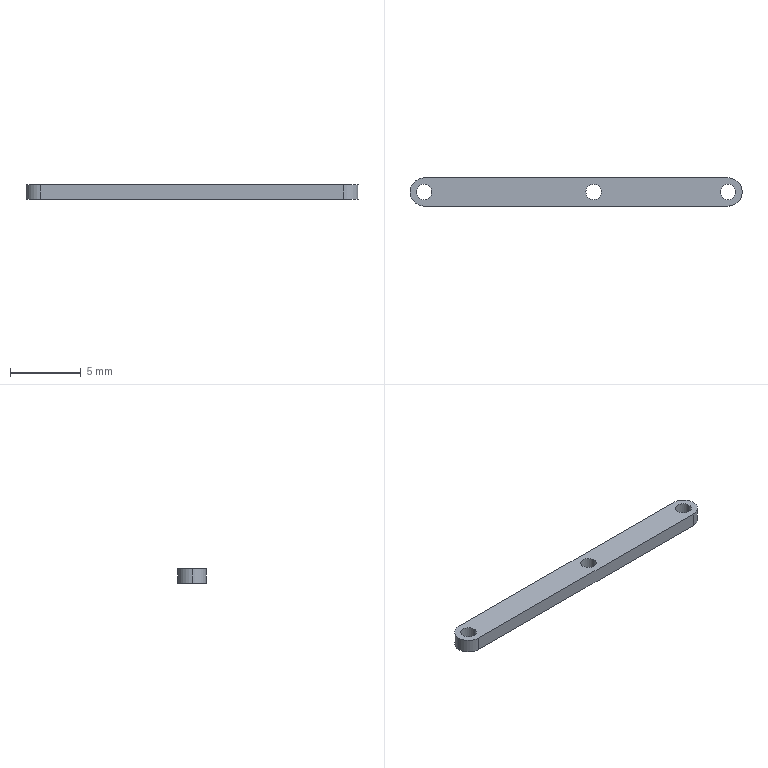Part | SolidWorks | features Extrusion 1, ICE 1 | 1 solid | 13 faces | box 23.5 x 2 x 1 mm | volume 43.291 mm3 | cylinder 9 | plane 4 | commonest cylinder face diameters 1.1 x6 2 x3
STEP:
#1=CARTESIAN_POINT('',(0.7,0.,0.5));
#2=VERTEX_POINT('',#1);
#3=CARTESIAN_POINT('',(1.8,0.,0.5));
#4=VERTEX_POINT('',#3);
#5=CARTESIAN_POINT('',(1.25,0.,0.5));
#6=DIRECTION('',(0.,0.,1.));
#7=DIRECTION('',(1.,0.,0.));
#8=AXIS2_PLACEMENT_3D('',#5,#6,#7);
#9=CIRCLE('',#8,0.55);
#10=EDGE_CURVE('',#2,#4,#9,.T.);
#11=ORIENTED_EDGE('',*,*,#10,.T.);
#12=CARTESIAN_POINT('',(1.8,0.,-0.5));
#13=VERTEX_POINT('',#12);
#14=CARTESIAN_POINT('',(1.8,0.,0.5));
#15=DIRECTION('',(0.,0.,-1.));
#16=VECTOR('',#15,1000.);
#17=LINE('',#14,#16);
#18=EDGE_CURVE('',#4,#13,#17,.T.);
#19=ORIENTED_EDGE('',*,*,#18,.T.);
#20=CARTESIAN_POINT('',(0.7,0.,-0.5));
#21=VERTEX_POINT('',#20);
#22=CARTESIAN_POINT('',(1.25,0.,-0.5));
#23=DIRECTION('',(0.,0.,1.));
#24=DIRECTION('',(1.,0.,0.));
#25=AXIS2_PLACEMENT_3D('',#22,#23,#24);
#26=CIRCLE('',#25,0.55);
#27=EDGE_CURVE('',#21,#13,#26,.T.);
#28=ORIENTED_EDGE('',*,*,#27,.F.);
#29=CARTESIAN_POINT('',(0.7,0.,0.5));
#30=DIRECTION('',(0.,0.,-1.));
#31=VECTOR('',#30,1000.);
#32=LINE('',#29,#31);
#33=EDGE_CURVE('',#2,#21,#32,.T.);
#34=ORIENTED_EDGE('',*,*,#33,.F.);
#35=EDGE_LOOP('',(#11,#19,#28,#34));
#36=FACE_OUTER_BOUND('',#35,.T.);
#37=CARTESIAN_POINT('',(1.25,0.,0.5));
#38=DIRECTION('',(0.,0.,-1.));
#39=DIRECTION('',(-1.,0.,0.));
#40=AXIS2_PLACEMENT_3D('',#37,#38,#39);
#41=CYLINDRICAL_SURFACE('',#40,0.55);
#42=ADVANCED_FACE('',(#36),#41,.F.);
#43=CARTESIAN_POINT('',(10.2,0.,0.5));
#44=VERTEX_POINT('',#43);
#45=CARTESIAN_POINT('',(11.3,0.,0.5));
#46=VERTEX_POINT('',#45);
#47=CARTESIAN_POINT('',(10.75,0.,0.5));
#48=DIRECTION('',(0.,0.,1.));
#49=DIRECTION('',(1.,0.,0.));
#50=AXIS2_PLACEMENT_3D('',#47,#48,#49);
#51=CIRCLE('',#50,0.55);
#52=EDGE_CURVE('',#44,#46,#51,.T.);
#53=ORIENTED_EDGE('',*,*,#52,.T.);
#54=CARTESIAN_POINT('',(11.3,0.,-0.5));
#55=VERTEX_POINT('',#54);
#56=CARTESIAN_POINT('',(11.3,0.,0.5));
#57=DIRECTION('',(0.,0.,-1.));
#58=VECTOR('',#57,1000.);
#59=LINE('',#56,#58);
#60=EDGE_CURVE('',#46,#55,#59,.T.);
#61=ORIENTED_EDGE('',*,*,#60,.T.);
#62=CARTESIAN_POINT('',(10.2,0.,-0.5));
#63=VERTEX_POINT('',#62);
#64=CARTESIAN_POINT('',(10.75,0.,-0.5));
#65=DIRECTION('',(0.,0.,1.));
#66=DIRECTION('',(1.,0.,0.));
#67=AXIS2_PLACEMENT_3D('',#64,#65,#66);
#68=CIRCLE('',#67,0.55);
#69=EDGE_CURVE('',#63,#55,#68,.T.);
#70=ORIENTED_EDGE('',*,*,#69,.F.);
#71=CARTESIAN_POINT('',(10.2,0.,0.5));
#72=DIRECTION('',(0.,0.,-1.));
#73=VECTOR('',#72,1000.);
#74=LINE('',#71,#73);
#75=EDGE_CURVE('',#44,#63,#74,.T.);
#76=ORIENTED_EDGE('',*,*,#75,.F.);
#77=EDGE_LOOP('',(#53,#61,#70,#76));
#78=FACE_OUTER_BOUND('',#77,.T.);
#79=CARTESIAN_POINT('',(10.75,0.,0.5));
#80=DIRECTION('',(0.,0.,-1.));
#81=DIRECTION('',(-1.,0.,0.));
#82=AXIS2_PLACEMENT_3D('',#79,#80,#81);
#83=CYLINDRICAL_SURFACE('',#82,0.55);
#84=ADVANCED_FACE('',(#78),#83,.F.);
#85=CARTESIAN_POINT('',(-11.3,0.,0.5));
#86=VERTEX_POINT('',#85);
#87=CARTESIAN_POINT('',(-10.2,0.,0.5));
#88=VERTEX_POINT('',#87);
#89=CARTESIAN_POINT('',(-10.75,0.,0.5));
#90=DIRECTION('',(0.,0.,1.));
#91=DIRECTION('',(1.,0.,0.));
#92=AXIS2_PLACEMENT_3D('',#89,#90,#91);
#93=CIRCLE('',#92,0.55);
#94=EDGE_CURVE('',#86,#88,#93,.T.);
#95=ORIENTED_EDGE('',*,*,#94,.T.);
#96=CARTESIAN_POINT('',(-10.2,0.,-0.5));
#97=VERTEX_POINT('',#96);
#98=CARTESIAN_POINT('',(-10.2,0.,0.5));
#99=DIRECTION('',(0.,0.,-1.));
#100=VECTOR('',#99,1000.);
#101=LINE('',#98,#100);
#102=EDGE_CURVE('',#88,#97,#101,.T.);
#103=ORIENTED_EDGE('',*,*,#102,.T.);
#104=CARTESIAN_POINT('',(-11.3,0.,-0.5));
#105=VERTEX_POINT('',#104);
#106=CARTESIAN_POINT('',(-10.75,0.,-0.5));
#107=DIRECTION('',(0.,0.,1.));
#108=DIRECTION('',(1.,0.,0.));
#109=AXIS2_PLACEMENT_3D('',#106,#107,#108);
#110=CIRCLE('',#109,0.55);
#111=EDGE_CURVE('',#105,#97,#110,.T.);
#112=ORIENTED_EDGE('',*,*,#111,.F.);
#113=CARTESIAN_POINT('',(-11.3,0.,0.5));
#114=DIRECTION('',(0.,0.,-1.));
#115=VECTOR('',#114,1000.);
#116=LINE('',#113,#115);
#117=EDGE_CURVE('',#86,#105,#116,.T.);
#118=ORIENTED_EDGE('',*,*,#117,.F.);
#119=EDGE_LOOP('',(#95,#103,#112,#118));
#120=FACE_OUTER_BOUND('',#119,.T.);
#121=CARTESIAN_POINT('',(-10.75,0.,0.5));
#122=DIRECTION('',(0.,0.,-1.));
#123=DIRECTION('',(-1.,0.,0.));
#124=AXIS2_PLACEMENT_3D('',#121,#122,#123);
#125=CYLINDRICAL_SURFACE('',#124,0.55);
#126=ADVANCED_FACE('',(#120),#125,.F.);
#127=CARTESIAN_POINT('',(-11.75,0.,0.5));
#128=VERTEX_POINT('',#127);
#129=CARTESIAN_POINT('',(-10.75,-1.,0.5));
#130=VERTEX_POINT('',#129);
#131=CARTESIAN_POINT('',(-10.75,0.,0.5));
#132=DIRECTION('',(0.,0.,1.));
#133=DIRECTION('',(1.,0.,0.));
#134=AXIS2_PLACEMENT_3D('',#131,#132,#133);
#135=CIRCLE('',#134,1.);
#136=EDGE_CURVE('',#128,#130,#135,.T.);
#137=ORIENTED_EDGE('',*,*,#136,.F.);
#138=CARTESIAN_POINT('',(-11.75,0.,-0.5));
#139=VERTEX_POINT('',#138);
#140=CARTESIAN_POINT('',(-11.75,0.,0.5));
#141=DIRECTION('',(0.,0.,-1.));
#142=VECTOR('',#141,1000.);
#143=LINE('',#140,#142);
#144=EDGE_CURVE('',#128,#139,#143,.T.);
#145=ORIENTED_EDGE('',*,*,#144,.T.);
#146=CARTESIAN_POINT('',(-10.75,-1.,-0.5));
#147=VERTEX_POINT('',#146);
#148=CARTESIAN_POINT('',(-10.75,0.,-0.5));
#149=DIRECTION('',(0.,0.,1.));
#150=DIRECTION('',(1.,0.,0.));
#151=AXIS2_PLACEMENT_3D('',#148,#149,#150);
#152=CIRCLE('',#151,1.);
#153=EDGE_CURVE('',#139,#147,#152,.T.);
#154=ORIENTED_EDGE('',*,*,#153,.T.);
#155=CARTESIAN_POINT('',(-10.75,-1.,0.5));
#156=DIRECTION('',(0.,0.,-1.));
#157=VECTOR('',#156,1000.);
#158=LINE('',#155,#157);
#159=EDGE_CURVE('',#130,#147,#158,.T.);
#160=ORIENTED_EDGE('',*,*,#159,.F.);
#161=EDGE_LOOP('',(#137,#145,#154,#160));
#162=FACE_OUTER_BOUND('',#161,.T.);
#163=CARTESIAN_POINT('',(-10.75,0.,0.5));
#164=DIRECTION('',(0.,0.,-1.));
#165=DIRECTION('',(-1.,0.,0.));
#166=AXIS2_PLACEMENT_3D('',#163,#164,#165);
#167=CYLINDRICAL_SURFACE('',#166,1.);
#168=ADVANCED_FACE('',(#162),#167,.T.);
#169=ORIENTED_EDGE('',*,*,#52,.F.);
#170=CARTESIAN_POINT('',(10.75,0.,0.5));
#171=DIRECTION('',(0.,0.,1.));
#172=DIRECTION('',(1.,0.,0.));
#173=AXIS2_PLACEMENT_3D('',#170,#171,#172);
#174=CIRCLE('',#173,0.55);
#175=EDGE_CURVE('',#46,#44,#174,.T.);
#176=ORIENTED_EDGE('',*,*,#175,.F.);
#177=EDGE_LOOP('',(#169,#176));
#178=FACE_BOUND('',#177,.T.);
#179=CARTESIAN_POINT('',(-10.75,1.,0.5));
#180=VERTEX_POINT('',#179);
#181=CARTESIAN_POINT('',(-10.75,0.,0.5));
#182=DIRECTION('',(0.,0.,1.));
#183=DIRECTION('',(1.,0.,0.));
#184=AXIS2_PLACEMENT_3D('',#181,#182,#183);
#185=CIRCLE('',#184,1.);
#186=EDGE_CURVE('',#180,#128,#185,.T.);
#187=ORIENTED_EDGE('',*,*,#186,.T.);
#188=ORIENTED_EDGE('',*,*,#136,.T.);
#189=CARTESIAN_POINT('',(10.75,-1.,0.5));
#190=VERTEX_POINT('',#189);
#191=CARTESIAN_POINT('',(-10.75,-1.,0.5));
#192=DIRECTION('',(1.,0.,0.));
#193=VECTOR('',#192,1000.);
#194=LINE('',#191,#193);
#195=EDGE_CURVE('',#130,#190,#194,.T.);
#196=ORIENTED_EDGE('',*,*,#195,.T.);
#197=CARTESIAN_POINT('',(10.75,1.,0.5));
#198=VERTEX_POINT('',#197);
#199=CARTESIAN_POINT('',(10.75,0.,0.5));
#200=DIRECTION('',(0.,0.,1.));
#201=DIRECTION('',(1.,0.,0.));
#202=AXIS2_PLACEMENT_3D('',#199,#200,#201);
#203=CIRCLE('',#202,1.);
#204=EDGE_CURVE('',#190,#198,#203,.T.);
#205=ORIENTED_EDGE('',*,*,#204,.T.);
#206=CARTESIAN_POINT('',(-10.75,1.,0.5));
#207=DIRECTION('',(-1.,0.,0.));
#208=VECTOR('',#207,1000.);
#209=LINE('',#206,#208);
#210=EDGE_CURVE('',#198,#180,#209,.T.);
#211=ORIENTED_EDGE('',*,*,#210,.T.);
#212=EDGE_LOOP('',(#187,#188,#196,#205,#211));
#213=FACE_OUTER_BOUND('',#212,.T.);
#214=ORIENTED_EDGE('',*,*,#94,.F.);
#215=CARTESIAN_POINT('',(-10.75,0.,0.5));
#216=DIRECTION('',(0.,0.,1.));
#217=DIRECTION('',(1.,0.,0.));
#218=AXIS2_PLACEMENT_3D('',#215,#216,#217);
#219=CIRCLE('',#218,0.55);
#220=EDGE_CURVE('',#88,#86,#219,.T.);
#221=ORIENTED_EDGE('',*,*,#220,.F.);
#222=EDGE_LOOP('',(#214,#221));
#223=FACE_BOUND('',#222,.T.);
#224=ORIENTED_EDGE('',*,*,#10,.F.);
#225=CARTESIAN_POINT('',(1.25,0.,0.5));
#226=DIRECTION('',(0.,0.,1.));
#227=DIRECTION('',(1.,0.,0.));
#228=AXIS2_PLACEMENT_3D('',#225,#226,#227);
#229=CIRCLE('',#228,0.55);
#230=EDGE_CURVE('',#4,#2,#229,.T.);
#231=ORIENTED_EDGE('',*,*,#230,.F.);
#232=EDGE_LOOP('',(#224,#231));
#233=FACE_BOUND('',#232,.T.);
#234=CARTESIAN_POINT('',(-10.75,0.,0.5));
#235=DIRECTION('',(0.,0.,1.));
#236=DIRECTION('',(1.,0.,0.));
#237=AXIS2_PLACEMENT_3D('',#234,#235,#236);
#238=PLANE('',#237);
#239=ADVANCED_FACE('',(#178,#213,#223,#233),#238,.T.);
#240=CARTESIAN_POINT('',(-10.75,1.,-0.5));
#241=VERTEX_POINT('',#240);
#242=CARTESIAN_POINT('',(-10.75,0.,-0.5));
#243=DIRECTION('',(0.,0.,1.));
#244=DIRECTION('',(1.,0.,0.));
#245=AXIS2_PLACEMENT_3D('',#242,#243,#244);
#246=CIRCLE('',#245,1.);
#247=EDGE_CURVE('',#241,#139,#246,.T.);
#248=ORIENTED_EDGE('',*,*,#247,.F.);
#249=CARTESIAN_POINT('',(10.75,1.,-0.5));
#250=VERTEX_POINT('',#249);
#251=CARTESIAN_POINT('',(-10.75,1.,-0.5));
#252=DIRECTION('',(-1.,0.,0.));
#253=VECTOR('',#252,1000.);
#254=LINE('',#251,#253);
#255=EDGE_CURVE('',#250,#241,#254,.T.);
#256=ORIENTED_EDGE('',*,*,#255,.F.);
#257=CARTESIAN_POINT('',(10.75,-1.,-0.5));
#258=VERTEX_POINT('',#257);
#259=CARTESIAN_POINT('',(10.75,0.,-0.5));
#260=DIRECTION('',(0.,0.,1.));
#261=DIRECTION('',(1.,0.,0.));
#262=AXIS2_PLACEMENT_3D('',#259,#260,#261);
#263=CIRCLE('',#262,1.);
#264=EDGE_CURVE('',#258,#250,#263,.T.);
#265=ORIENTED_EDGE('',*,*,#264,.F.);
#266=CARTESIAN_POINT('',(-10.75,-1.,-0.5));
#267=DIRECTION('',(1.,0.,0.));
#268=VECTOR('',#267,1000.);
#269=LINE('',#266,#268);
#270=EDGE_CURVE('',#147,#258,#269,.T.);
#271=ORIENTED_EDGE('',*,*,#270,.F.);
#272=ORIENTED_EDGE('',*,*,#153,.F.);
#273=EDGE_LOOP('',(#248,#256,#265,#271,#272));
#274=FACE_OUTER_BOUND('',#273,.T.);
#275=ORIENTED_EDGE('',*,*,#111,.T.);
#276=CARTESIAN_POINT('',(-10.75,0.,-0.5));
#277=DIRECTION('',(0.,0.,1.));
#278=DIRECTION('',(1.,0.,0.));
#279=AXIS2_PLACEMENT_3D('',#276,#277,#278);
#280=CIRCLE('',#279,0.55);
#281=EDGE_CURVE('',#97,#105,#280,.T.);
#282=ORIENTED_EDGE('',*,*,#281,.T.);
#283=EDGE_LOOP('',(#275,#282));
#284=FACE_BOUND('',#283,.T.);
#285=ORIENTED_EDGE('',*,*,#69,.T.);
#286=CARTESIAN_POINT('',(10.75,0.,-0.5));
#287=DIRECTION('',(0.,0.,1.));
#288=DIRECTION('',(1.,0.,0.));
#289=AXIS2_PLACEMENT_3D('',#286,#287,#288);
#290=CIRCLE('',#289,0.55);
#291=EDGE_CURVE('',#55,#63,#290,.T.);
#292=ORIENTED_EDGE('',*,*,#291,.T.);
#293=EDGE_LOOP('',(#285,#292));
#294=FACE_BOUND('',#293,.T.);
#295=ORIENTED_EDGE('',*,*,#27,.T.);
#296=CARTESIAN_POINT('',(1.25,0.,-0.5));
#297=DIRECTION('',(0.,0.,1.));
#298=DIRECTION('',(1.,0.,0.));
#299=AXIS2_PLACEMENT_3D('',#296,#297,#298);
#300=CIRCLE('',#299,0.55);
#301=EDGE_CURVE('',#13,#21,#300,.T.);
#302=ORIENTED_EDGE('',*,*,#301,.T.);
#303=EDGE_LOOP('',(#295,#302));
#304=FACE_BOUND('',#303,.T.);
#305=CARTESIAN_POINT('',(-10.75,0.,-0.5));
#306=DIRECTION('',(0.,0.,1.));
#307=DIRECTION('',(1.,0.,0.));
#308=AXIS2_PLACEMENT_3D('',#305,#306,#307);
#309=PLANE('',#308);
#310=ADVANCED_FACE('',(#274,#284,#294,#304),#309,.F.);
#311=ORIENTED_EDGE('',*,*,#144,.F.);
#312=ORIENTED_EDGE('',*,*,#186,.F.);
#313=CARTESIAN_POINT('',(-10.75,1.,0.5));
#314=DIRECTION('',(0.,0.,-1.));
#315=VECTOR('',#314,1000.);
#316=LINE('',#313,#315);
#317=EDGE_CURVE('',#180,#241,#316,.T.);
#318=ORIENTED_EDGE('',*,*,#317,.T.);
#319=ORIENTED_EDGE('',*,*,#247,.T.);
#320=EDGE_LOOP('',(#311,#312,#318,#319));
#321=FACE_OUTER_BOUND('',#320,.T.);
#322=CARTESIAN_POINT('',(-10.75,0.,0.5));
#323=DIRECTION('',(0.,0.,-1.));
#324=DIRECTION('',(-1.,0.,0.));
#325=AXIS2_PLACEMENT_3D('',#322,#323,#324);
#326=CYLINDRICAL_SURFACE('',#325,1.);
#327=ADVANCED_FACE('',(#321),#326,.T.);
#328=ORIENTED_EDGE('',*,*,#270,.T.);
#329=CARTESIAN_POINT('',(10.75,-1.,0.5));
#330=DIRECTION('',(0.,0.,-1.));
#331=VECTOR('',#330,1000.);
#332=LINE('',#329,#331);
#333=EDGE_CURVE('',#190,#258,#332,.T.);
#334=ORIENTED_EDGE('',*,*,#333,.F.);
#335=ORIENTED_EDGE('',*,*,#195,.F.);
#336=ORIENTED_EDGE('',*,*,#159,.T.);
#337=EDGE_LOOP('',(#328,#334,#335,#336));
#338=FACE_OUTER_BOUND('',#337,.T.);
#339=CARTESIAN_POINT('',(-10.75,-1.,0.5));
#340=DIRECTION('',(0.,1.,0.));
#341=DIRECTION('',(-1.,0.,0.));
#342=AXIS2_PLACEMENT_3D('',#339,#340,#341);
#343=PLANE('',#342);
#344=ADVANCED_FACE('',(#338),#343,.F.);
#345=ORIENTED_EDGE('',*,*,#264,.T.);
#346=CARTESIAN_POINT('',(10.75,1.,0.5));
#347=DIRECTION('',(0.,0.,-1.));
#348=VECTOR('',#347,1000.);
#349=LINE('',#346,#348);
#350=EDGE_CURVE('',#198,#250,#349,.T.);
#351=ORIENTED_EDGE('',*,*,#350,.F.);
#352=ORIENTED_EDGE('',*,*,#204,.F.);
#353=ORIENTED_EDGE('',*,*,#333,.T.);
#354=EDGE_LOOP('',(#345,#351,#352,#353));
#355=FACE_OUTER_BOUND('',#354,.T.);
#356=CARTESIAN_POINT('',(10.75,0.,0.5));
#357=DIRECTION('',(0.,0.,-1.));
#358=DIRECTION('',(-1.,0.,0.));
#359=AXIS2_PLACEMENT_3D('',#356,#357,#358);
#360=CYLINDRICAL_SURFACE('',#359,1.);
#361=ADVANCED_FACE('',(#355),#360,.T.);
#362=ORIENTED_EDGE('',*,*,#255,.T.);
#363=ORIENTED_EDGE('',*,*,#317,.F.);
#364=ORIENTED_EDGE('',*,*,#210,.F.);
#365=ORIENTED_EDGE('',*,*,#350,.T.);
#366=EDGE_LOOP('',(#362,#363,#364,#365));
#367=FACE_OUTER_BOUND('',#366,.T.);
#368=CARTESIAN_POINT('',(-10.75,1.,0.5));
#369=DIRECTION('',(0.,-1.,0.));
#370=DIRECTION('',(1.,0.,0.));
#371=AXIS2_PLACEMENT_3D('',#368,#369,#370);
#372=PLANE('',#371);
#373=ADVANCED_FACE('',(#367),#372,.F.);
#374=ORIENTED_EDGE('',*,*,#102,.F.);
#375=ORIENTED_EDGE('',*,*,#220,.T.);
#376=ORIENTED_EDGE('',*,*,#117,.T.);
#377=ORIENTED_EDGE('',*,*,#281,.F.);
#378=EDGE_LOOP('',(#374,#375,#376,#377));
#379=FACE_OUTER_BOUND('',#378,.T.);
#380=CARTESIAN_POINT('',(-10.75,0.,0.5));
#381=DIRECTION('',(0.,0.,-1.));
#382=DIRECTION('',(-1.,0.,0.));
#383=AXIS2_PLACEMENT_3D('',#380,#381,#382);
#384=CYLINDRICAL_SURFACE('',#383,0.55);
#385=ADVANCED_FACE('',(#379),#384,.F.);
#386=ORIENTED_EDGE('',*,*,#60,.F.);
#387=ORIENTED_EDGE('',*,*,#175,.T.);
#388=ORIENTED_EDGE('',*,*,#75,.T.);
#389=ORIENTED_EDGE('',*,*,#291,.F.);
#390=EDGE_LOOP('',(#386,#387,#388,#389));
#391=FACE_OUTER_BOUND('',#390,.T.);
#392=CARTESIAN_POINT('',(10.75,0.,0.5));
#393=DIRECTION('',(0.,0.,-1.));
#394=DIRECTION('',(-1.,0.,0.));
#395=AXIS2_PLACEMENT_3D('',#392,#393,#394);
#396=CYLINDRICAL_SURFACE('',#395,0.55);
#397=ADVANCED_FACE('',(#391),#396,.F.);
#398=ORIENTED_EDGE('',*,*,#18,.F.);
#399=ORIENTED_EDGE('',*,*,#230,.T.);
#400=ORIENTED_EDGE('',*,*,#33,.T.);
#401=ORIENTED_EDGE('',*,*,#301,.F.);
#402=EDGE_LOOP('',(#398,#399,#400,#401));
#403=FACE_OUTER_BOUND('',#402,.T.);
#404=CARTESIAN_POINT('',(1.25,0.,0.5));
#405=DIRECTION('',(0.,0.,-1.));
#406=DIRECTION('',(-1.,0.,0.));
#407=AXIS2_PLACEMENT_3D('',#404,#405,#406);
#408=CYLINDRICAL_SURFACE('',#407,0.55);
#409=ADVANCED_FACE('',(#403),#408,.F.);
#410=CLOSED_SHELL('',(#42,#84,#126,#168,#239,#310,#327,#344,#361,#373,#385,#397,#409));
#411=MANIFOLD_SOLID_BREP('',#410);
#412=CARTESIAN_POINT('',(0.,0.,0.));
#413=DIRECTION('',(0.,0.,1.));
#414=DIRECTION('',(1.,0.,0.));
#415=AXIS2_PLACEMENT_3D('',#412,#413,#414);
#416=(LENGTH_UNIT()NAMED_UNIT(*)SI_UNIT(.MILLI.,.METRE.));
#417=UNCERTAINTY_MEASURE_WITH_UNIT(LENGTH_MEASURE(0.00001),#416,'','');
#418=(NAMED_UNIT(*)PLANE_ANGLE_UNIT()SI_UNIT($,.RADIAN.));
#419=(NAMED_UNIT(*)SI_UNIT($,.STERADIAN.)SOLID_ANGLE_UNIT());
#420=(GEOMETRIC_REPRESENTATION_CONTEXT(3)GLOBAL_UNCERTAINTY_ASSIGNED_CONTEXT((#417))GLOBAL_UNIT_ASSIGNED_CONTEXT((#416,#418,#419))REPRESENTATION_CONTEXT('',''));
#421=ADVANCED_BREP_SHAPE_REPRESENTATION('',(#411,#415),#420);